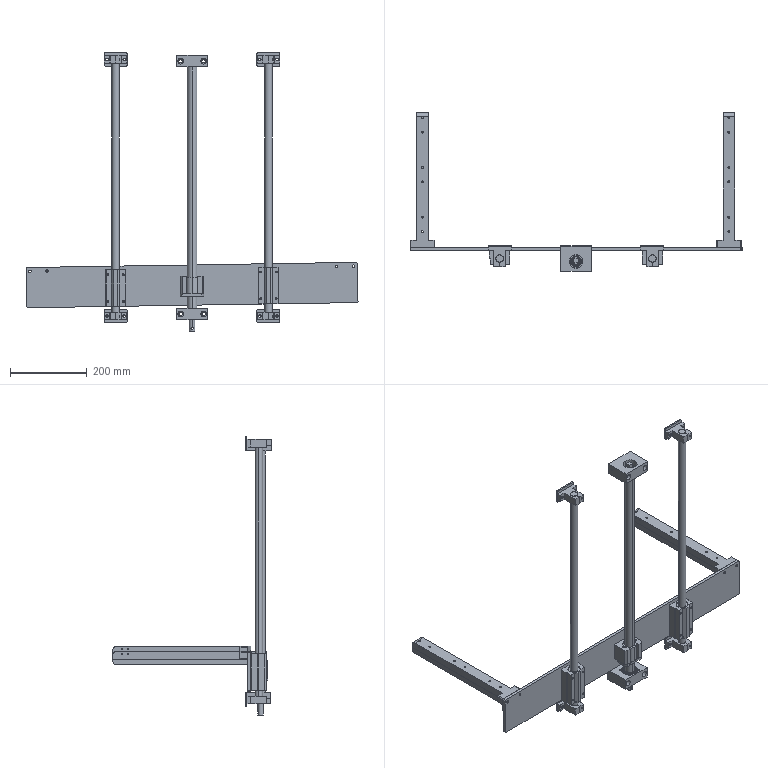Part | SolidWorks | features MirrorCompFeat 1, ReferencePattern 1 | 24 solids | 934 faces | box 866.479 x 413.5 x 727.5 mm | volume 3012478 mm3 | cylinder 383 | plane 287 | cone 150 | spline 114 | commonest cylinder face diameters 5 x48 6.6 x44 20 x34 4.2 x32 1 x24 9 x24